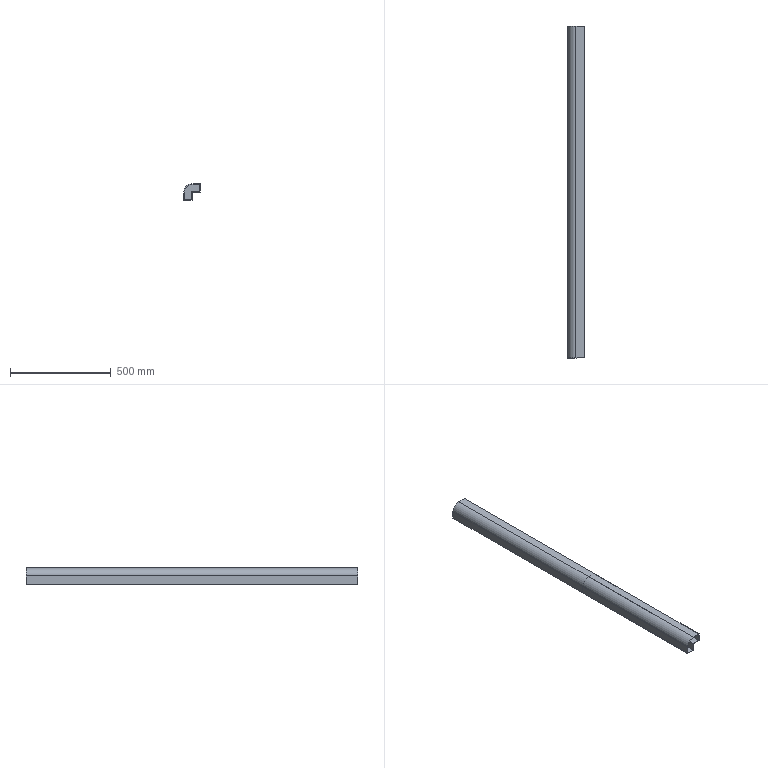Part | 1 solid | 17 faces | box 80 x 1650 x 80 mm | volume 4500258 mm3 | plane 15 | cylinder 2 | commonest cylinder face diameters 76 x1 80 x1
STEP:
#1=CARTESIAN_POINT('',(-580.,528.,602.));
#2=VERTEX_POINT('',#1);
#3=CARTESIAN_POINT('',(-580.,-210.,602.));
#4=VERTEX_POINT('',#3);
#5=CARTESIAN_POINT('',(-580.,514.1,602.));
#6=DIRECTION('',(0.,-1.,0.));
#7=VECTOR('',#6,1000.);
#8=LINE('',#5,#7);
#9=EDGE_CURVE('',#2,#4,#8,.T.);
#10=ORIENTED_EDGE('',*,*,#9,.F.);
#11=CARTESIAN_POINT('',(-580.,528.,562.));
#12=VERTEX_POINT('',#11);
#13=CARTESIAN_POINT('',(-580.,528.,562.));
#14=DIRECTION('',(0.,0.,1.));
#15=VECTOR('',#14,1000.);
#16=LINE('',#13,#15);
#17=EDGE_CURVE('',#12,#2,#16,.T.);
#18=ORIENTED_EDGE('',*,*,#17,.F.);
#19=CARTESIAN_POINT('',(-580.,-210.,562.));
#20=VERTEX_POINT('',#19);
#21=CARTESIAN_POINT('',(-580.,2.,562.));
#22=DIRECTION('',(0.,1.,0.));
#23=VECTOR('',#22,1000.);
#24=LINE('',#21,#23);
#25=EDGE_CURVE('',#20,#12,#24,.T.);
#26=ORIENTED_EDGE('',*,*,#25,.F.);
#27=CARTESIAN_POINT('',(-580.,-210.,636.9));
#28=DIRECTION('',(0.,0.,-1.));
#29=VECTOR('',#28,1000.);
#30=LINE('',#27,#29);
#31=EDGE_CURVE('',#4,#20,#30,.T.);
#32=ORIENTED_EDGE('',*,*,#31,.F.);
#33=EDGE_LOOP('',(#10,#18,#26,#32));
#34=FACE_OUTER_BOUND('',#33,.T.);
#35=CARTESIAN_POINT('',(-580.,514.1,636.9));
#36=DIRECTION('',(1.,0.,0.));
#37=DIRECTION('',(0.,0.,-1.));
#38=AXIS2_PLACEMENT_3D('',#35,#36,#37);
#39=PLANE('',#38);
#40=ADVANCED_FACE('',(#34),#39,.F.);
#41=CARTESIAN_POINT('',(-540.,-210.,638.));
#42=VERTEX_POINT('',#41);
#43=CARTESIAN_POINT('',(-578.,-210.,638.));
#44=VERTEX_POINT('',#43);
#45=CARTESIAN_POINT('',(-540.,-210.,638.));
#46=DIRECTION('',(-1.,0.,0.));
#47=VECTOR('',#46,1000.);
#48=LINE('',#45,#47);
#49=EDGE_CURVE('',#42,#44,#48,.T.);
#50=ORIENTED_EDGE('',*,*,#49,.F.);
#51=CARTESIAN_POINT('',(-540.,-210.,602.));
#52=VERTEX_POINT('',#51);
#53=CARTESIAN_POINT('',(-540.,-210.,638.));
#54=DIRECTION('',(0.,0.,-1.));
#55=VECTOR('',#54,1000.);
#56=LINE('',#53,#55);
#57=EDGE_CURVE('',#42,#52,#56,.T.);
#58=ORIENTED_EDGE('',*,*,#57,.T.);
#59=CARTESIAN_POINT('',(-580.,-210.,602.));
#60=DIRECTION('',(1.,0.,0.));
#61=VECTOR('',#60,1000.);
#62=LINE('',#59,#61);
#63=EDGE_CURVE('',#4,#52,#62,.T.);
#64=ORIENTED_EDGE('',*,*,#63,.F.);
#65=ORIENTED_EDGE('',*,*,#31,.T.);
#66=CARTESIAN_POINT('',(-616.,-210.,562.));
#67=VERTEX_POINT('',#66);
#68=CARTESIAN_POINT('',(-616.,-210.,562.));
#69=DIRECTION('',(1.,0.,0.));
#70=VECTOR('',#69,1000.);
#71=LINE('',#68,#70);
#72=EDGE_CURVE('',#67,#20,#71,.T.);
#73=ORIENTED_EDGE('',*,*,#72,.F.);
#74=CARTESIAN_POINT('',(-616.,-210.,600.));
#75=VERTEX_POINT('',#74);
#76=CARTESIAN_POINT('',(-616.,-210.,636.9));
#77=DIRECTION('',(0.,0.,-1.));
#78=VECTOR('',#77,1000.);
#79=LINE('',#76,#78);
#80=EDGE_CURVE('',#75,#67,#79,.T.);
#81=ORIENTED_EDGE('',*,*,#80,.F.);
#82=CARTESIAN_POINT('',(-578.,-210.,600.));
#83=DIRECTION('',(0.,1.,0.));
#84=DIRECTION('',(1.,0.,0.));
#85=AXIS2_PLACEMENT_3D('',#82,#83,#84);
#86=CIRCLE('',#85,38.);
#87=EDGE_CURVE('',#75,#44,#86,.T.);
#88=ORIENTED_EDGE('',*,*,#87,.T.);
#89=EDGE_LOOP('',(#50,#58,#64,#65,#73,#81,#88));
#90=FACE_BOUND('',#89,.T.);
#91=CARTESIAN_POINT('',(-538.,-210.,600.));
#92=VERTEX_POINT('',#91);
#93=CARTESIAN_POINT('',(-538.,-210.,640.));
#94=VERTEX_POINT('',#93);
#95=CARTESIAN_POINT('',(-538.,-210.,565.1));
#96=DIRECTION('',(0.,0.,1.));
#97=VECTOR('',#96,1000.);
#98=LINE('',#95,#97);
#99=EDGE_CURVE('',#92,#94,#98,.T.);
#100=ORIENTED_EDGE('',*,*,#99,.T.);
#101=CARTESIAN_POINT('',(-578.,-210.,640.));
#102=VERTEX_POINT('',#101);
#103=CARTESIAN_POINT('',(-618.,-210.,640.));
#104=DIRECTION('',(1.,0.,0.));
#105=VECTOR('',#104,1000.);
#106=LINE('',#103,#105);
#107=EDGE_CURVE('',#102,#94,#106,.T.);
#108=ORIENTED_EDGE('',*,*,#107,.F.);
#109=CARTESIAN_POINT('',(-618.,-210.,600.));
#110=VERTEX_POINT('',#109);
#111=CARTESIAN_POINT('',(-578.,-210.,600.));
#112=DIRECTION('',(0.,-1.,0.));
#113=DIRECTION('',(1.,0.,0.));
#114=AXIS2_PLACEMENT_3D('',#111,#112,#113);
#115=CIRCLE('',#114,40.);
#116=EDGE_CURVE('',#102,#110,#115,.T.);
#117=ORIENTED_EDGE('',*,*,#116,.T.);
#118=CARTESIAN_POINT('',(-618.,-210.,560.));
#119=VERTEX_POINT('',#118);
#120=CARTESIAN_POINT('',(-618.,-210.,565.1));
#121=DIRECTION('',(0.,0.,1.));
#122=VECTOR('',#121,1000.);
#123=LINE('',#120,#122);
#124=EDGE_CURVE('',#119,#110,#123,.T.);
#125=ORIENTED_EDGE('',*,*,#124,.F.);
#126=CARTESIAN_POINT('',(-578.,-210.,560.));
#127=VERTEX_POINT('',#126);
#128=CARTESIAN_POINT('',(-618.,-210.,560.));
#129=DIRECTION('',(-1.,0.,0.));
#130=VECTOR('',#129,1000.);
#131=LINE('',#128,#130);
#132=EDGE_CURVE('',#127,#119,#131,.T.);
#133=ORIENTED_EDGE('',*,*,#132,.F.);
#134=CARTESIAN_POINT('',(-578.,-210.,600.));
#135=VERTEX_POINT('',#134);
#136=CARTESIAN_POINT('',(-578.,-210.,600.));
#137=DIRECTION('',(0.,0.,-1.));
#138=VECTOR('',#137,1000.);
#139=LINE('',#136,#138);
#140=EDGE_CURVE('',#135,#127,#139,.T.);
#141=ORIENTED_EDGE('',*,*,#140,.F.);
#142=CARTESIAN_POINT('',(-538.,-210.,600.));
#143=DIRECTION('',(-1.,0.,0.));
#144=VECTOR('',#143,1000.);
#145=LINE('',#142,#144);
#146=EDGE_CURVE('',#92,#135,#145,.T.);
#147=ORIENTED_EDGE('',*,*,#146,.F.);
#148=EDGE_LOOP('',(#100,#108,#117,#125,#133,#141,#147));
#149=FACE_OUTER_BOUND('',#148,.T.);
#150=CARTESIAN_POINT('',(-618.,-210.,565.1));
#151=DIRECTION('',(0.,-1.,0.));
#152=DIRECTION('',(1.,0.,0.));
#153=AXIS2_PLACEMENT_3D('',#150,#151,#152);
#154=PLANE('',#153);
#155=ADVANCED_FACE('',(#90,#149),#154,.T.);
#156=CARTESIAN_POINT('',(-538.,1440.,640.));
#157=VERTEX_POINT('',#156);
#158=CARTESIAN_POINT('',(-538.,2.,640.));
#159=DIRECTION('',(0.,1.,0.));
#160=VECTOR('',#159,1000.);
#161=LINE('',#158,#160);
#162=EDGE_CURVE('',#94,#157,#161,.T.);
#163=ORIENTED_EDGE('',*,*,#162,.F.);
#164=ORIENTED_EDGE('',*,*,#99,.F.);
#165=CARTESIAN_POINT('',(-538.,1440.,600.));
#166=VERTEX_POINT('',#165);
#167=CARTESIAN_POINT('',(-538.,1440.,600.));
#168=DIRECTION('',(0.,-1.,0.));
#169=VECTOR('',#168,1000.);
#170=LINE('',#167,#169);
#171=EDGE_CURVE('',#166,#92,#170,.T.);
#172=ORIENTED_EDGE('',*,*,#171,.F.);
#173=CARTESIAN_POINT('',(-538.,1440.,565.1));
#174=DIRECTION('',(0.,0.,1.));
#175=VECTOR('',#174,1000.);
#176=LINE('',#173,#175);
#177=EDGE_CURVE('',#166,#157,#176,.T.);
#178=ORIENTED_EDGE('',*,*,#177,.T.);
#179=EDGE_LOOP('',(#163,#164,#172,#178));
#180=FACE_OUTER_BOUND('',#179,.T.);
#181=CARTESIAN_POINT('',(-538.,2.,565.1));
#182=DIRECTION('',(1.,0.,0.));
#183=DIRECTION('',(0.,0.,-1.));
#184=AXIS2_PLACEMENT_3D('',#181,#182,#183);
#185=PLANE('',#184);
#186=ADVANCED_FACE('',(#180),#185,.T.);
#187=ORIENTED_EDGE('',*,*,#107,.T.);
#188=ORIENTED_EDGE('',*,*,#162,.T.);
#189=CARTESIAN_POINT('',(-578.,1440.,640.));
#190=VERTEX_POINT('',#189);
#191=CARTESIAN_POINT('',(-538.,1440.,640.));
#192=DIRECTION('',(-1.,0.,0.));
#193=VECTOR('',#192,1000.);
#194=LINE('',#191,#193);
#195=EDGE_CURVE('',#157,#190,#194,.T.);
#196=ORIENTED_EDGE('',*,*,#195,.T.);
#197=CARTESIAN_POINT('',(-578.,0.,640.));
#198=DIRECTION('',(0.,-1.,0.));
#199=VECTOR('',#198,1000.);
#200=LINE('',#197,#199);
#201=EDGE_CURVE('',#190,#102,#200,.T.);
#202=ORIENTED_EDGE('',*,*,#201,.T.);
#203=EDGE_LOOP('',(#187,#188,#196,#202));
#204=FACE_OUTER_BOUND('',#203,.T.);
#205=CARTESIAN_POINT('',(0.,0.,640.));
#206=DIRECTION('',(0.,0.,1.));
#207=DIRECTION('',(1.,0.,0.));
#208=AXIS2_PLACEMENT_3D('',#205,#206,#207);
#209=PLANE('',#208);
#210=ADVANCED_FACE('',(#204),#209,.T.);
#211=ORIENTED_EDGE('',*,*,#124,.T.);
#212=CARTESIAN_POINT('',(-618.,1440.,600.));
#213=VERTEX_POINT('',#212);
#214=CARTESIAN_POINT('',(-618.,1440.,600.));
#215=DIRECTION('',(0.,1.,0.));
#216=VECTOR('',#215,1000.);
#217=LINE('',#214,#216);
#218=EDGE_CURVE('',#110,#213,#217,.T.);
#219=ORIENTED_EDGE('',*,*,#218,.T.);
#220=CARTESIAN_POINT('',(-618.,1440.,560.));
#221=VERTEX_POINT('',#220);
#222=CARTESIAN_POINT('',(-618.,1440.,565.1));
#223=DIRECTION('',(0.,0.,1.));
#224=VECTOR('',#223,1000.);
#225=LINE('',#222,#224);
#226=EDGE_CURVE('',#221,#213,#225,.T.);
#227=ORIENTED_EDGE('',*,*,#226,.F.);
#228=CARTESIAN_POINT('',(-618.,1440.,560.));
#229=DIRECTION('',(0.,1.,0.));
#230=VECTOR('',#229,1000.);
#231=LINE('',#228,#230);
#232=EDGE_CURVE('',#119,#221,#231,.T.);
#233=ORIENTED_EDGE('',*,*,#232,.F.);
#234=EDGE_LOOP('',(#211,#219,#227,#233));
#235=FACE_OUTER_BOUND('',#234,.T.);
#236=CARTESIAN_POINT('',(-618.,1440.,565.1));
#237=DIRECTION('',(-1.,0.,0.));
#238=DIRECTION('',(0.,-1.,0.));
#239=AXIS2_PLACEMENT_3D('',#236,#237,#238);
#240=PLANE('',#239);
#241=ADVANCED_FACE('',(#235),#240,.T.);
#242=ORIENTED_EDGE('',*,*,#226,.T.);
#243=CARTESIAN_POINT('',(-578.,1440.,600.));
#244=DIRECTION('',(0.,1.,0.));
#245=DIRECTION('',(0.,0.,1.));
#246=AXIS2_PLACEMENT_3D('',#243,#244,#245);
#247=CIRCLE('',#246,40.);
#248=EDGE_CURVE('',#213,#190,#247,.T.);
#249=ORIENTED_EDGE('',*,*,#248,.T.);
#250=ORIENTED_EDGE('',*,*,#195,.F.);
#251=ORIENTED_EDGE('',*,*,#177,.F.);
#252=CARTESIAN_POINT('',(-578.,1440.,600.));
#253=VERTEX_POINT('',#252);
#254=CARTESIAN_POINT('',(-538.,1440.,600.));
#255=DIRECTION('',(-1.,0.,0.));
#256=VECTOR('',#255,1000.);
#257=LINE('',#254,#256);
#258=EDGE_CURVE('',#166,#253,#257,.T.);
#259=ORIENTED_EDGE('',*,*,#258,.T.);
#260=CARTESIAN_POINT('',(-578.,1440.,560.));
#261=VERTEX_POINT('',#260);
#262=CARTESIAN_POINT('',(-578.,1440.,600.));
#263=DIRECTION('',(0.,0.,-1.));
#264=VECTOR('',#263,1000.);
#265=LINE('',#262,#264);
#266=EDGE_CURVE('',#253,#261,#265,.T.);
#267=ORIENTED_EDGE('',*,*,#266,.T.);
#268=CARTESIAN_POINT('',(-538.,1440.,560.));
#269=DIRECTION('',(1.,0.,0.));
#270=VECTOR('',#269,1000.);
#271=LINE('',#268,#270);
#272=EDGE_CURVE('',#221,#261,#271,.T.);
#273=ORIENTED_EDGE('',*,*,#272,.F.);
#274=EDGE_LOOP('',(#242,#249,#250,#251,#259,#267,#273));
#275=FACE_OUTER_BOUND('',#274,.T.);
#276=CARTESIAN_POINT('',(-538.,1440.,565.1));
#277=DIRECTION('',(0.,1.,0.));
#278=DIRECTION('',(0.,0.,1.));
#279=AXIS2_PLACEMENT_3D('',#276,#277,#278);
#280=PLANE('',#279);
#281=ADVANCED_FACE('',(#275),#280,.T.);
#282=ORIENTED_EDGE('',*,*,#132,.T.);
#283=ORIENTED_EDGE('',*,*,#232,.T.);
#284=ORIENTED_EDGE('',*,*,#272,.T.);
#285=CARTESIAN_POINT('',(-578.,1440.,560.));
#286=DIRECTION('',(0.,-1.,0.));
#287=VECTOR('',#286,1000.);
#288=LINE('',#285,#287);
#289=EDGE_CURVE('',#261,#127,#288,.T.);
#290=ORIENTED_EDGE('',*,*,#289,.T.);
#291=EDGE_LOOP('',(#282,#283,#284,#290));
#292=FACE_OUTER_BOUND('',#291,.T.);
#293=CARTESIAN_POINT('',(0.,0.,560.));
#294=DIRECTION('',(0.,0.,1.));
#295=DIRECTION('',(1.,0.,0.));
#296=AXIS2_PLACEMENT_3D('',#293,#294,#295);
#297=PLANE('',#296);
#298=ADVANCED_FACE('',(#292),#297,.F.);
#299=CARTESIAN_POINT('',(-616.,528.,600.));
#300=VERTEX_POINT('',#299);
#301=CARTESIAN_POINT('',(-616.,528.,562.));
#302=VERTEX_POINT('',#301);
#303=CARTESIAN_POINT('',(-616.,528.,638.));
#304=DIRECTION('',(0.,0.,-1.));
#305=VECTOR('',#304,1000.);
#306=LINE('',#303,#305);
#307=EDGE_CURVE('',#300,#302,#306,.T.);
#308=ORIENTED_EDGE('',*,*,#307,.F.);
#309=CARTESIAN_POINT('',(-616.,2.,600.));
#310=DIRECTION('',(0.,-1.,0.));
#311=VECTOR('',#310,1000.);
#312=LINE('',#309,#311);
#313=EDGE_CURVE('',#300,#75,#312,.T.);
#314=ORIENTED_EDGE('',*,*,#313,.T.);
#315=ORIENTED_EDGE('',*,*,#80,.T.);
#316=CARTESIAN_POINT('',(-616.,528.,562.));
#317=DIRECTION('',(0.,-1.,0.));
#318=VECTOR('',#317,1000.);
#319=LINE('',#316,#318);
#320=EDGE_CURVE('',#302,#67,#319,.T.);
#321=ORIENTED_EDGE('',*,*,#320,.F.);
#322=EDGE_LOOP('',(#308,#314,#315,#321));
#323=FACE_OUTER_BOUND('',#322,.T.);
#324=CARTESIAN_POINT('',(-616.,2.,636.9));
#325=DIRECTION('',(-1.,0.,0.));
#326=DIRECTION('',(0.,0.,1.));
#327=AXIS2_PLACEMENT_3D('',#324,#325,#326);
#328=PLANE('',#327);
#329=ADVANCED_FACE('',(#323),#328,.F.);
#330=ORIENTED_EDGE('',*,*,#57,.F.);
#331=CARTESIAN_POINT('',(-540.,528.,638.));
#332=VERTEX_POINT('',#331);
#333=CARTESIAN_POINT('',(-540.,505.9,638.));
#334=DIRECTION('',(0.,-1.,0.));
#335=VECTOR('',#334,1000.);
#336=LINE('',#333,#335);
#337=EDGE_CURVE('',#332,#42,#336,.T.);
#338=ORIENTED_EDGE('',*,*,#337,.F.);
#339=CARTESIAN_POINT('',(-540.,528.,602.));
#340=VERTEX_POINT('',#339);
#341=CARTESIAN_POINT('',(-540.,528.,602.));
#342=DIRECTION('',(0.,0.,1.));
#343=VECTOR('',#342,1000.);
#344=LINE('',#341,#343);
#345=EDGE_CURVE('',#340,#332,#344,.T.);
#346=ORIENTED_EDGE('',*,*,#345,.F.);
#347=CARTESIAN_POINT('',(-540.,2.,602.));
#348=DIRECTION('',(0.,1.,0.));
#349=VECTOR('',#348,1000.);
#350=LINE('',#347,#349);
#351=EDGE_CURVE('',#52,#340,#350,.T.);
#352=ORIENTED_EDGE('',*,*,#351,.F.);
#353=EDGE_LOOP('',(#330,#338,#346,#352));
#354=FACE_OUTER_BOUND('',#353,.T.);
#355=CARTESIAN_POINT('',(-540.,15.9,638.));
#356=DIRECTION('',(1.,0.,0.));
#357=DIRECTION('',(0.,0.,-1.));
#358=AXIS2_PLACEMENT_3D('',#355,#356,#357);
#359=PLANE('',#358);
#360=ADVANCED_FACE('',(#354),#359,.F.);
#361=ORIENTED_EDGE('',*,*,#337,.T.);
#362=ORIENTED_EDGE('',*,*,#49,.T.);
#363=CARTESIAN_POINT('',(-578.,528.,638.));
#364=VERTEX_POINT('',#363);
#365=CARTESIAN_POINT('',(-578.,0.,638.));
#366=DIRECTION('',(0.,1.,0.));
#367=VECTOR('',#366,1000.);
#368=LINE('',#365,#367);
#369=EDGE_CURVE('',#44,#364,#368,.T.);
#370=ORIENTED_EDGE('',*,*,#369,.T.);
#371=CARTESIAN_POINT('',(-540.,528.,638.));
#372=DIRECTION('',(-1.,0.,0.));
#373=VECTOR('',#372,1000.);
#374=LINE('',#371,#373);
#375=EDGE_CURVE('',#332,#364,#374,.T.);
#376=ORIENTED_EDGE('',*,*,#375,.F.);
#377=EDGE_LOOP('',(#361,#362,#370,#376));
#378=FACE_OUTER_BOUND('',#377,.T.);
#379=CARTESIAN_POINT('',(0.,0.,638.));
#380=DIRECTION('',(0.,0.,-1.));
#381=DIRECTION('',(-1.,0.,0.));
#382=AXIS2_PLACEMENT_3D('',#379,#380,#381);
#383=PLANE('',#382);
#384=ADVANCED_FACE('',(#378),#383,.T.);
#385=ORIENTED_EDGE('',*,*,#320,.T.);
#386=ORIENTED_EDGE('',*,*,#72,.T.);
#387=ORIENTED_EDGE('',*,*,#25,.T.);
#388=CARTESIAN_POINT('',(-616.,528.,562.));
#389=DIRECTION('',(1.,0.,0.));
#390=VECTOR('',#389,1000.);
#391=LINE('',#388,#390);
#392=EDGE_CURVE('',#302,#12,#391,.T.);
#393=ORIENTED_EDGE('',*,*,#392,.F.);
#394=EDGE_LOOP('',(#385,#386,#387,#393));
#395=FACE_OUTER_BOUND('',#394,.T.);
#396=CARTESIAN_POINT('',(0.,0.,562.));
#397=DIRECTION('',(0.,0.,1.));
#398=DIRECTION('',(1.,0.,0.));
#399=AXIS2_PLACEMENT_3D('',#396,#397,#398);
#400=PLANE('',#399);
#401=ADVANCED_FACE('',(#395),#400,.T.);
#402=ORIENTED_EDGE('',*,*,#351,.T.);
#403=CARTESIAN_POINT('',(-580.,528.,602.));
#404=DIRECTION('',(1.,0.,0.));
#405=VECTOR('',#404,1000.);
#406=LINE('',#403,#405);
#407=EDGE_CURVE('',#2,#340,#406,.T.);
#408=ORIENTED_EDGE('',*,*,#407,.F.);
#409=ORIENTED_EDGE('',*,*,#9,.T.);
#410=ORIENTED_EDGE('',*,*,#63,.T.);
#411=EDGE_LOOP('',(#402,#408,#409,#410));
#412=FACE_OUTER_BOUND('',#411,.T.);
#413=CARTESIAN_POINT('',(0.,0.,602.));
#414=DIRECTION('',(0.,0.,1.));
#415=DIRECTION('',(1.,0.,0.));
#416=AXIS2_PLACEMENT_3D('',#413,#414,#415);
#417=PLANE('',#416);
#418=ADVANCED_FACE('',(#412),#417,.T.);
#419=ORIENTED_EDGE('',*,*,#375,.T.);
#420=CARTESIAN_POINT('',(-578.,528.,600.));
#421=DIRECTION('',(0.,-1.,0.));
#422=DIRECTION('',(0.,0.,-1.));
#423=AXIS2_PLACEMENT_3D('',#420,#421,#422);
#424=CIRCLE('',#423,38.);
#425=EDGE_CURVE('',#364,#300,#424,.T.);
#426=ORIENTED_EDGE('',*,*,#425,.T.);
#427=ORIENTED_EDGE('',*,*,#307,.T.);
#428=ORIENTED_EDGE('',*,*,#392,.T.);
#429=ORIENTED_EDGE('',*,*,#17,.T.);
#430=ORIENTED_EDGE('',*,*,#407,.T.);
#431=ORIENTED_EDGE('',*,*,#345,.T.);
#432=EDGE_LOOP('',(#419,#426,#427,#428,#429,#430,#431));
#433=FACE_OUTER_BOUND('',#432,.T.);
#434=CARTESIAN_POINT('',(0.,528.,0.));
#435=DIRECTION('',(0.,-1.,0.));
#436=DIRECTION('',(0.,0.,-1.));
#437=AXIS2_PLACEMENT_3D('',#434,#435,#436);
#438=PLANE('',#437);
#439=ADVANCED_FACE('',(#433),#438,.T.);
#440=ORIENTED_EDGE('',*,*,#140,.T.);
#441=ORIENTED_EDGE('',*,*,#289,.F.);
#442=ORIENTED_EDGE('',*,*,#266,.F.);
#443=CARTESIAN_POINT('',(-578.,1440.,600.));
#444=DIRECTION('',(0.,-1.,0.));
#445=VECTOR('',#444,1000.);
#446=LINE('',#443,#445);
#447=EDGE_CURVE('',#253,#135,#446,.T.);
#448=ORIENTED_EDGE('',*,*,#447,.T.);
#449=EDGE_LOOP('',(#440,#441,#442,#448));
#450=FACE_OUTER_BOUND('',#449,.T.);
#451=CARTESIAN_POINT('',(-578.,1440.,600.));
#452=DIRECTION('',(-1.,0.,0.));
#453=DIRECTION('',(0.,-1.,0.));
#454=AXIS2_PLACEMENT_3D('',#451,#452,#453);
#455=PLANE('',#454);
#456=ADVANCED_FACE('',(#450),#455,.F.);
#457=ORIENTED_EDGE('',*,*,#146,.T.);
#458=ORIENTED_EDGE('',*,*,#447,.F.);
#459=ORIENTED_EDGE('',*,*,#258,.F.);
#460=ORIENTED_EDGE('',*,*,#171,.T.);
#461=EDGE_LOOP('',(#457,#458,#459,#460));
#462=FACE_OUTER_BOUND('',#461,.T.);
#463=CARTESIAN_POINT('',(-538.,1440.,600.));
#464=DIRECTION('',(0.,0.,1.));
#465=DIRECTION('',(1.,0.,0.));
#466=AXIS2_PLACEMENT_3D('',#463,#464,#465);
#467=PLANE('',#466);
#468=ADVANCED_FACE('',(#462),#467,.F.);
#469=ORIENTED_EDGE('',*,*,#87,.F.);
#470=ORIENTED_EDGE('',*,*,#313,.F.);
#471=ORIENTED_EDGE('',*,*,#425,.F.);
#472=ORIENTED_EDGE('',*,*,#369,.F.);
#473=EDGE_LOOP('',(#469,#470,#471,#472));
#474=FACE_OUTER_BOUND('',#473,.T.);
#475=CARTESIAN_POINT('',(-578.,0.,600.));
#476=DIRECTION('',(0.,1.,0.));
#477=DIRECTION('',(0.,0.,1.));
#478=AXIS2_PLACEMENT_3D('',#475,#476,#477);
#479=CYLINDRICAL_SURFACE('',#478,38.);
#480=ADVANCED_FACE('',(#474),#479,.F.);
#481=ORIENTED_EDGE('',*,*,#248,.F.);
#482=ORIENTED_EDGE('',*,*,#218,.F.);
#483=ORIENTED_EDGE('',*,*,#116,.F.);
#484=ORIENTED_EDGE('',*,*,#201,.F.);
#485=EDGE_LOOP('',(#481,#482,#483,#484));
#486=FACE_OUTER_BOUND('',#485,.T.);
#487=CARTESIAN_POINT('',(-578.,0.,600.));
#488=DIRECTION('',(0.,-1.,0.));
#489=DIRECTION('',(1.,0.,0.));
#490=AXIS2_PLACEMENT_3D('',#487,#488,#489);
#491=CYLINDRICAL_SURFACE('',#490,40.);
#492=ADVANCED_FACE('',(#486),#491,.T.);
#493=CLOSED_SHELL('',(#40,#155,#186,#210,#241,#281,#298,#329,#360,#384,#401,#418,#439,#456,#468,#480,#492));
#494=MANIFOLD_SOLID_BREP('',#493);
#495=CARTESIAN_POINT('',(0.,0.,0.));
#496=DIRECTION('',(0.,0.,1.));
#497=DIRECTION('',(1.,0.,0.));
#498=AXIS2_PLACEMENT_3D('',#495,#496,#497);
#499=(LENGTH_UNIT()NAMED_UNIT(*)SI_UNIT(.MILLI.,.METRE.));
#500=UNCERTAINTY_MEASURE_WITH_UNIT(LENGTH_MEASURE(0.00001),#499,'','');
#501=(NAMED_UNIT(*)PLANE_ANGLE_UNIT()SI_UNIT($,.RADIAN.));
#502=(NAMED_UNIT(*)SI_UNIT($,.STERADIAN.)SOLID_ANGLE_UNIT());
#503=(GEOMETRIC_REPRESENTATION_CONTEXT(3)GLOBAL_UNCERTAINTY_ASSIGNED_CONTEXT((#500))GLOBAL_UNIT_ASSIGNED_CONTEXT((#499,#501,#502))REPRESENTATION_CONTEXT('',''));
#504=ADVANCED_BREP_SHAPE_REPRESENTATION('',(#494,#498),#503);